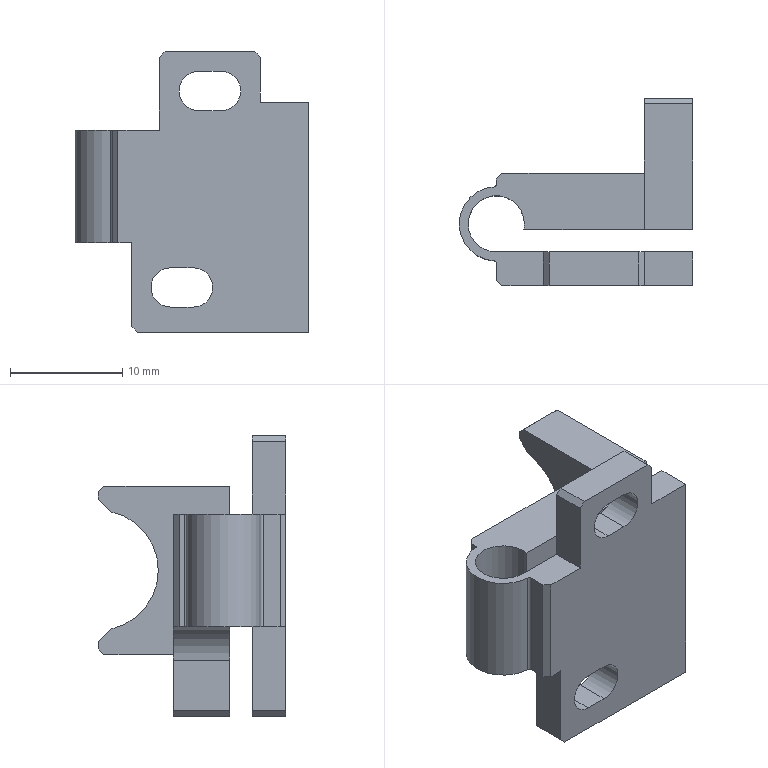Part | SolidWorks | features MoveFace 8, Chamfer 5, ICE 5, BaseBody 1, DelFace 1, Fillet 1 | 1 solid | 55 faces | box 20.78 x 16.7 x 25 mm | volume 2347 mm3 | plane 38 | cylinder 17 | commonest cylinder face diameters 3.5 x6 5 x3 0.4 x2 3.75 x2 6 x1 6.6 x1